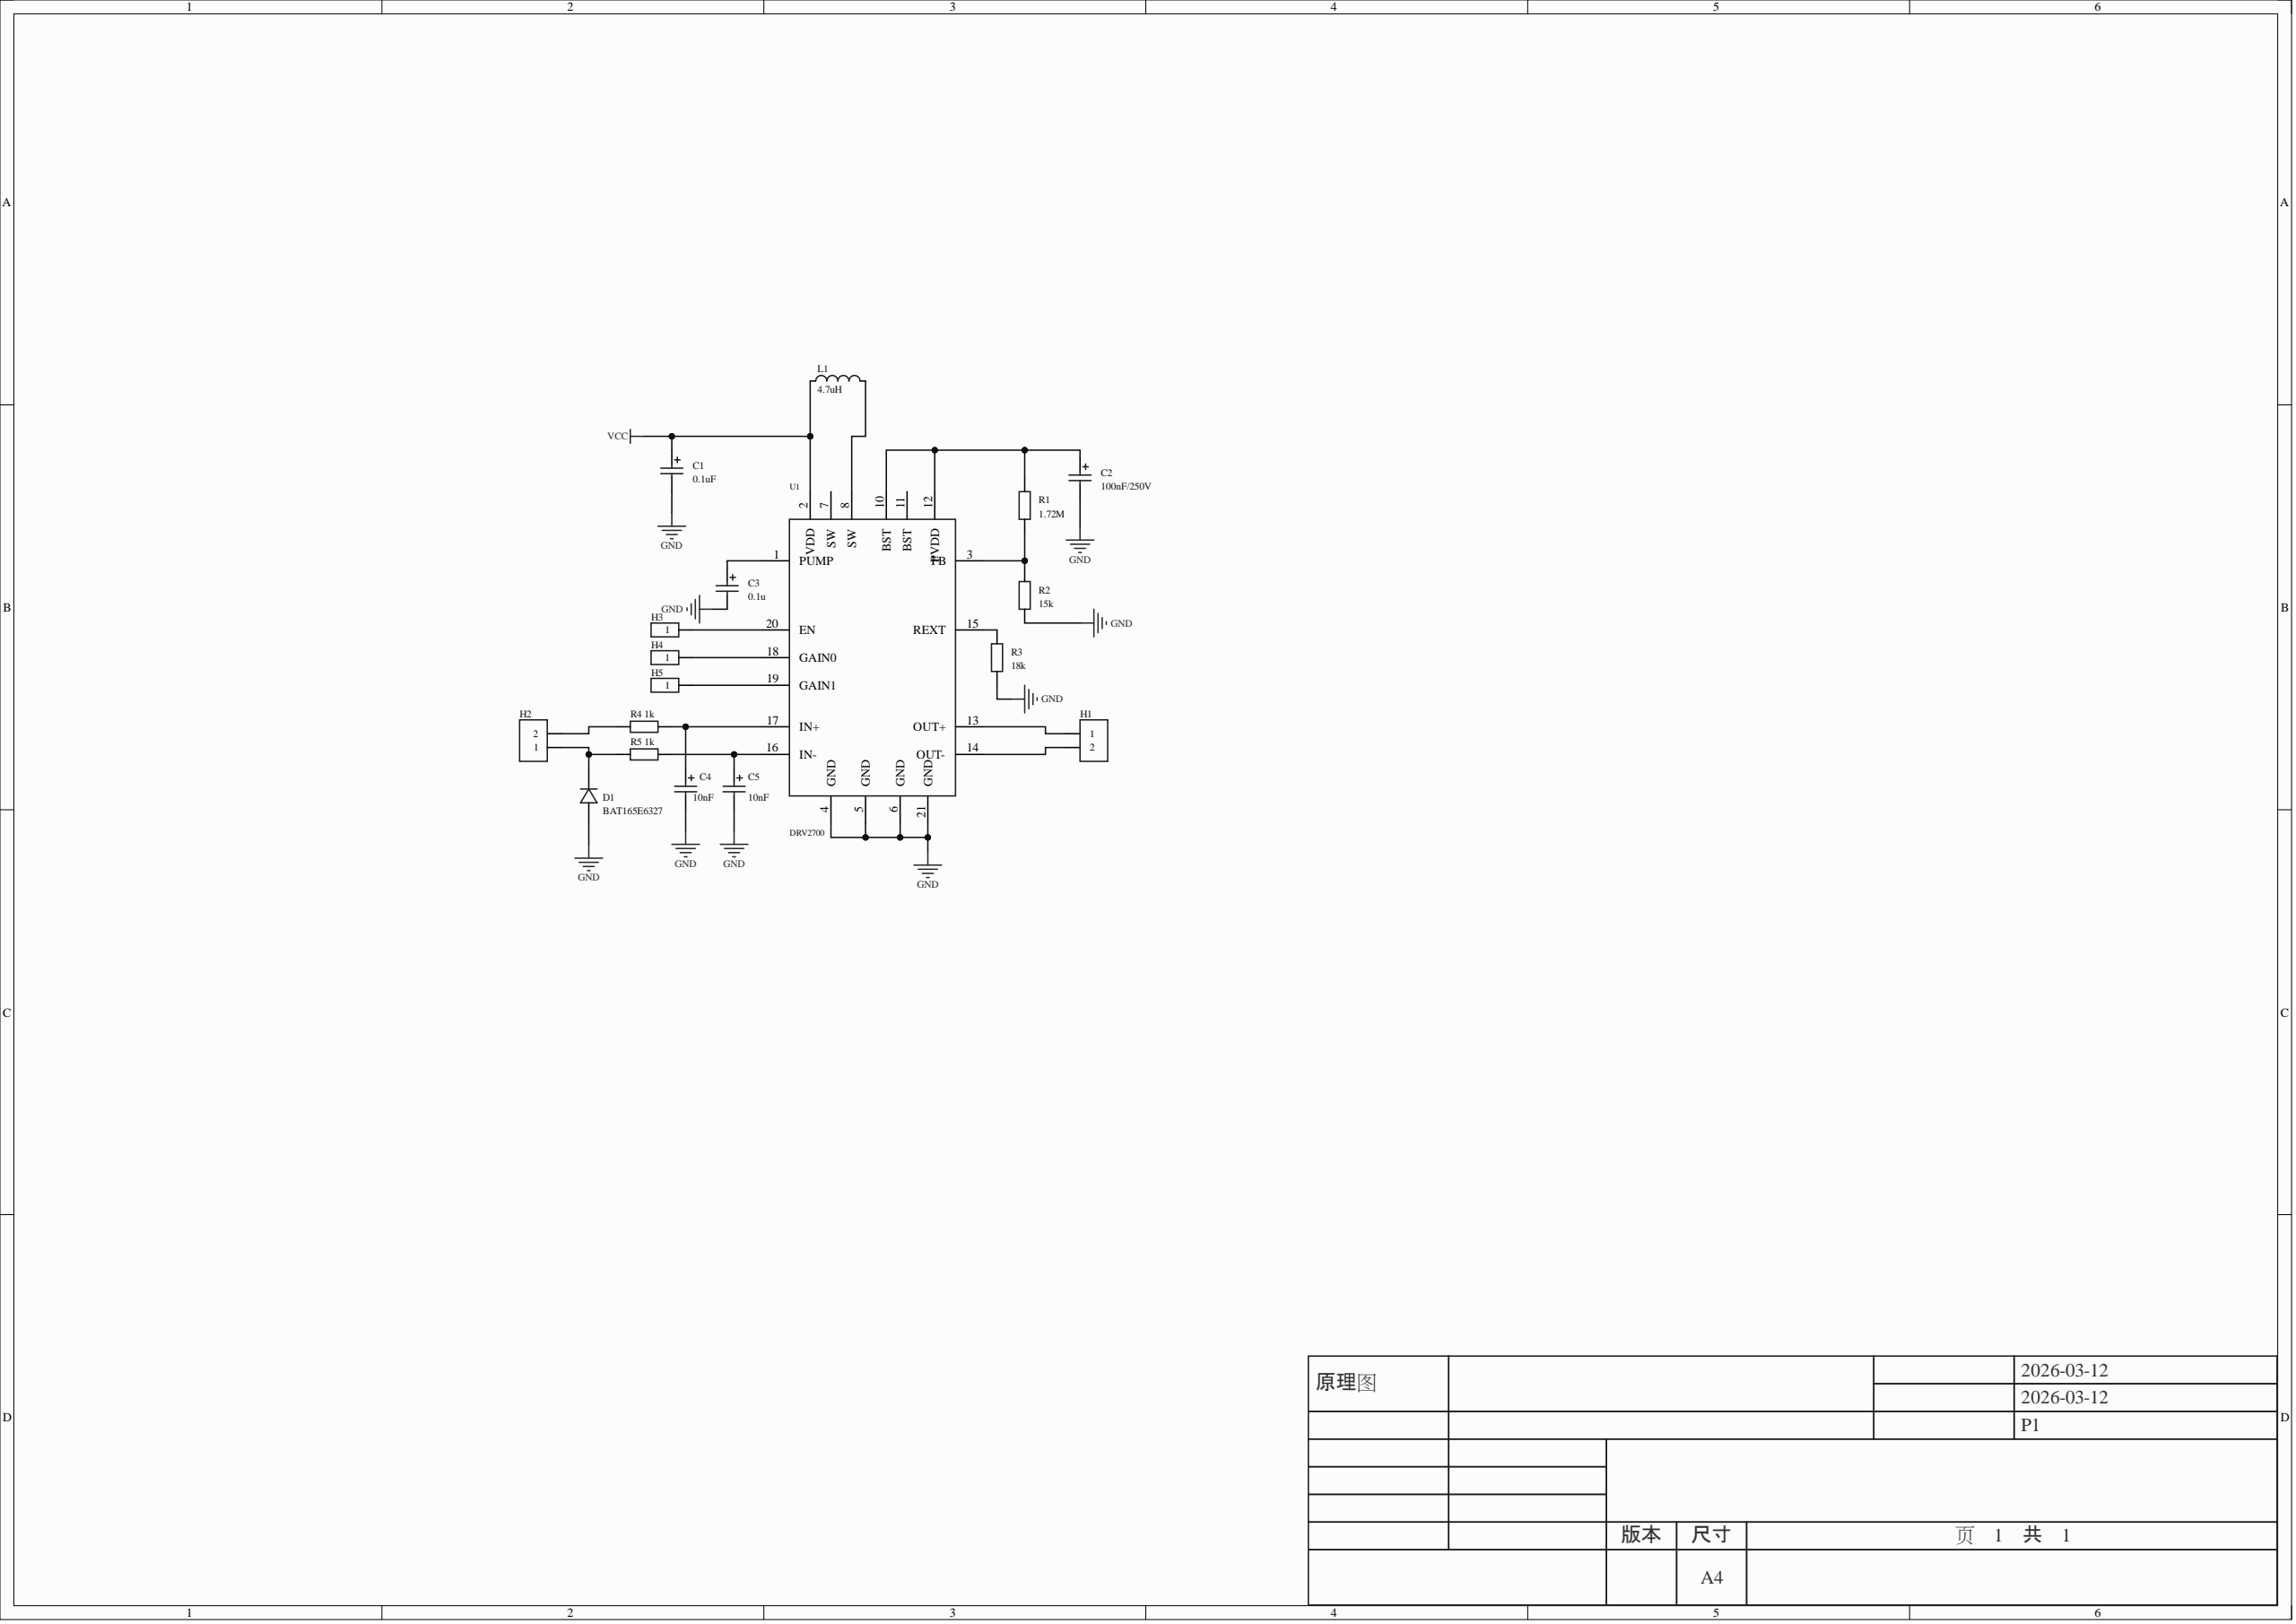Circuit board | Altium Designer | 18 parts | 16 nets
Bill of materials:
Comment,Description,Designator,Footprint,LibRef,Quantity
"0.1uF","","C1","C_Ele_SMD_3x5.4mm","C_Ele_SMD_3x5.4mm","1"
"100nF/250V","","C2","C_Ele_SMD_3x5.4mm","C_Ele_SMD_3x5.4mm","1"
"0.1u","","C3","C_Ele_SMD_3x5.4mm","C_Ele_SMD_3x5.4mm","1"
"10nF","","C4, C5","C_Ele_SMD_3x5.4mm","C_Ele_SMD_3x5.4mm","2"
"BAT165E6327","二极管配置:1个独立式;正向压降(Vf):740mV@750mA;直流反向耐压(Vr):40V;整流电流:750mA;","D1","SOD-323_L1.8-W1.3-LS2.5-RD","BAT165E6327","1"
"","","H1, H2","HDR-TH_2P-P2.54-V-F","HDR-F_2.54_1x2P","2"
"","","H3, H4, H5","HDR-TH_1P-V-M_XKB_X4611WV-01I-C28D40","HDR-M_2.54_1x1P","3"
"4.7uH","电感值:4.7uH;精度:±20%;额定电流:3A;饱和电流(Isat):3.5A;类型:一体成型电感;","L1","IND-SMD_L4.6-W4.1-A","SRG0420-4R7-M","1"
"1.72M","","R1","Res_1W","Res_AXIAL-1W","1"
"15k","","R2","Res_1W","Res_AXIAL-1W","1"
"18k","","R3","Res_1W","Res_AXIAL-1W","1"
"1k","","R4, R5","Res_1W","Res_AXIAL-1W","2"
"DRV2700","","U1","TI-RGP20-2700X2700TP_V","DRV2700","1"
Netlist (Protel format):
[
C1
C_Ele_SMD_3x5.4mm
0.1uF



]
[
C2
C_Ele_SMD_3x5.4mm
100nF/250V



]
[
C3
C_Ele_SMD_3x5.4mm
0.1u



]
[
C4
C_Ele_SMD_3x5.4mm
10nF



]
[
C5
C_Ele_SMD_3x5.4mm
10nF



]
[
D1
SOD-323_L1.8-W1.3-LS2.5-RD
BAT165E6327



]
[
H1
HDR-TH_2P-P2.54-V-F




]
[
H2
HDR-TH_2P-P2.54-V-F




]
[
H3
HDR-TH_1P-V-M_XKB_X4611WV-01I-C28D40




]
[
H4
HDR-TH_1P-V-M_XKB_X4611WV-01I-C28D40




]
[
H5
HDR-TH_1P-V-M_XKB_X4611WV-01I-C28D40




]
[
L1
IND-SMD_L4.6-W4.1-A
4.7uH



]
[
R1
Res_1W
1.72M



]
[
R2
Res_1W
15k



]
[
R3
Res_1W
18k



]
[
R4
Res_1W
1k



]
[
R5
Res_1W
1k



]
[
U1
TI-RGP20-2700X2700TP_V
DRV2700



]
(
VCC
C1-1
L1-1
U1-2
)
(
NetR3_2
R3-2
U1-15
)
(
NetR1_1
R1-1
R2-2
U1-3
)
(
NetL1_2
L1-2
U1-8
)
(
NetH5_1
H5-1
U1-19
)
(
NetH4_1
H4-1
U1-18
)
(
NetH3_1
H3-1
U1-20
)
(
NetH2_2
H2-2
R4-1
)
(
NetH1_2
H1-2
U1-14
)
(
NetH1_1
H1-1
U1-13
)
(
NetD1_1
D1-1
H2-1
R5-1
)
(
NetC5_1
C5-1
R5-2
U1-16
)
(
NetC4_1
C4-1
R4-2
U1-17
)
(
NetC3_1
C3-1
U1-1
)
(
NetC2_1
C2-1
R1-2
U1-10
U1-12
)
(
GND
C1-2
C2-2
C3-2
C4-2
C5-2
D1-2
R2-1
R3-1
U1-4
U1-5
U1-6
U1-21
)